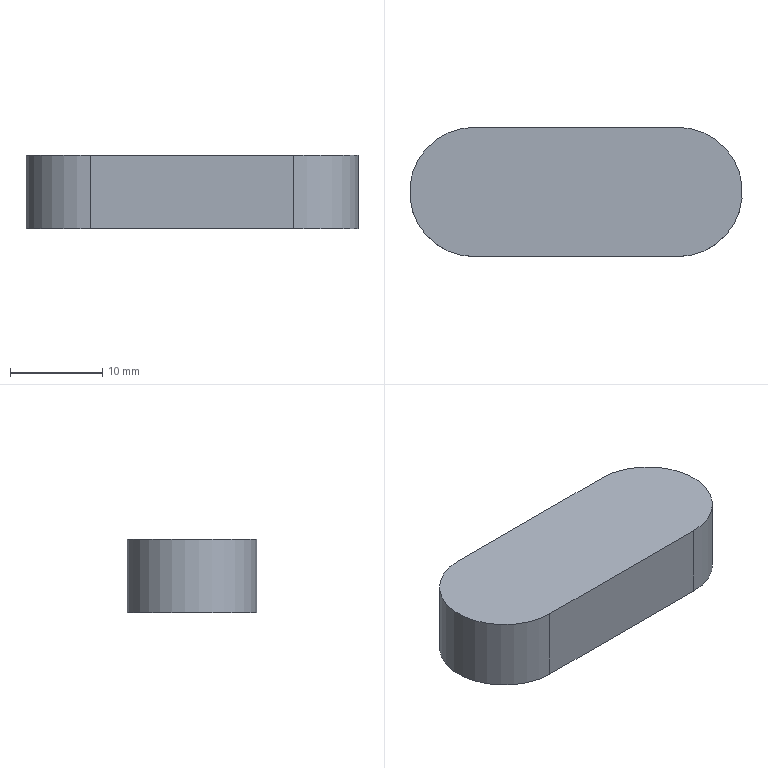Part | NX | features DATUM_CSYS 2, EXTRUDE 1, SKETCH 1 | 1 solid | 6 faces | box 36 x 14 x 8 mm | volume 3696 mm3 | plane 4 | cylinder 2 | commonest cylinder face diameters 14 x2
STEP:
#1=CARTESIAN_POINT('',(-11.,-7.,0.));
#2=VERTEX_POINT('',#1);
#3=CARTESIAN_POINT('',(11.,-7.,0.));
#4=VERTEX_POINT('',#3);
#5=CARTESIAN_POINT('',(-11.,-7.,0.));
#6=DIRECTION('',(1.,0.,0.));
#7=VECTOR('',#6,1000.);
#8=LINE('',#5,#7);
#9=EDGE_CURVE('',#2,#4,#8,.T.);
#10=ORIENTED_EDGE('',*,*,#9,.T.);
#11=CARTESIAN_POINT('',(11.,-7.,8.));
#12=VERTEX_POINT('',#11);
#13=CARTESIAN_POINT('',(11.,-7.,8.));
#14=DIRECTION('',(0.,0.,-1.));
#15=VECTOR('',#14,1000.);
#16=LINE('',#13,#15);
#17=EDGE_CURVE('',#12,#4,#16,.T.);
#18=ORIENTED_EDGE('',*,*,#17,.F.);
#19=CARTESIAN_POINT('',(-11.,-7.,8.));
#20=VERTEX_POINT('',#19);
#21=CARTESIAN_POINT('',(-11.,-7.,8.));
#22=DIRECTION('',(1.,0.,0.));
#23=VECTOR('',#22,1000.);
#24=LINE('',#21,#23);
#25=EDGE_CURVE('',#20,#12,#24,.T.);
#26=ORIENTED_EDGE('',*,*,#25,.F.);
#27=CARTESIAN_POINT('',(-11.,-7.,8.));
#28=DIRECTION('',(0.,0.,-1.));
#29=VECTOR('',#28,1000.);
#30=LINE('',#27,#29);
#31=EDGE_CURVE('',#20,#2,#30,.T.);
#32=ORIENTED_EDGE('',*,*,#31,.T.);
#33=EDGE_LOOP('',(#10,#18,#26,#32));
#34=FACE_BOUND('',#33,.T.);
#35=CARTESIAN_POINT('',(-11.,-7.,8.));
#36=DIRECTION('',(0.,1.,0.));
#37=DIRECTION('',(0.,0.,1.));
#38=AXIS2_PLACEMENT_3D('',#35,#36,#37);
#39=PLANE('',#38);
#40=ADVANCED_FACE('',(#34),#39,.F.);
#41=CARTESIAN_POINT('',(11.,7.,0.));
#42=VERTEX_POINT('',#41);
#43=CARTESIAN_POINT('',(11.,0.,0.));
#44=DIRECTION('',(0.,0.,1.));
#45=DIRECTION('',(-1.,0.,0.));
#46=AXIS2_PLACEMENT_3D('',#43,#44,#45);
#47=CIRCLE('',#46,7.);
#48=EDGE_CURVE('',#4,#42,#47,.T.);
#49=ORIENTED_EDGE('',*,*,#48,.T.);
#50=CARTESIAN_POINT('',(11.,7.,8.));
#51=VERTEX_POINT('',#50);
#52=CARTESIAN_POINT('',(11.,7.,8.));
#53=DIRECTION('',(0.,0.,-1.));
#54=VECTOR('',#53,1000.);
#55=LINE('',#52,#54);
#56=EDGE_CURVE('',#51,#42,#55,.T.);
#57=ORIENTED_EDGE('',*,*,#56,.F.);
#58=CARTESIAN_POINT('',(11.,0.,8.));
#59=DIRECTION('',(0.,0.,1.));
#60=DIRECTION('',(-1.,0.,0.));
#61=AXIS2_PLACEMENT_3D('',#58,#59,#60);
#62=CIRCLE('',#61,7.);
#63=EDGE_CURVE('',#12,#51,#62,.T.);
#64=ORIENTED_EDGE('',*,*,#63,.F.);
#65=ORIENTED_EDGE('',*,*,#17,.T.);
#66=EDGE_LOOP('',(#49,#57,#64,#65));
#67=FACE_BOUND('',#66,.T.);
#68=CARTESIAN_POINT('',(11.,0.,8.));
#69=DIRECTION('',(0.,0.,-1.));
#70=DIRECTION('',(-1.,0.,0.));
#71=AXIS2_PLACEMENT_3D('',#68,#69,#70);
#72=CYLINDRICAL_SURFACE('',#71,7.);
#73=ADVANCED_FACE('',(#67),#72,.T.);
#74=CARTESIAN_POINT('',(-11.,7.,0.));
#75=VERTEX_POINT('',#74);
#76=CARTESIAN_POINT('',(11.,7.,0.));
#77=DIRECTION('',(-1.,0.,0.));
#78=VECTOR('',#77,1000.);
#79=LINE('',#76,#78);
#80=EDGE_CURVE('',#42,#75,#79,.T.);
#81=ORIENTED_EDGE('',*,*,#80,.T.);
#82=CARTESIAN_POINT('',(-11.,7.,8.));
#83=VERTEX_POINT('',#82);
#84=CARTESIAN_POINT('',(-11.,7.,8.));
#85=DIRECTION('',(0.,0.,-1.));
#86=VECTOR('',#85,1000.);
#87=LINE('',#84,#86);
#88=EDGE_CURVE('',#83,#75,#87,.T.);
#89=ORIENTED_EDGE('',*,*,#88,.F.);
#90=CARTESIAN_POINT('',(11.,7.,8.));
#91=DIRECTION('',(-1.,0.,0.));
#92=VECTOR('',#91,1000.);
#93=LINE('',#90,#92);
#94=EDGE_CURVE('',#51,#83,#93,.T.);
#95=ORIENTED_EDGE('',*,*,#94,.F.);
#96=ORIENTED_EDGE('',*,*,#56,.T.);
#97=EDGE_LOOP('',(#81,#89,#95,#96));
#98=FACE_BOUND('',#97,.T.);
#99=CARTESIAN_POINT('',(11.,7.,8.));
#100=DIRECTION('',(0.,-1.,0.));
#101=DIRECTION('',(0.,0.,-1.));
#102=AXIS2_PLACEMENT_3D('',#99,#100,#101);
#103=PLANE('',#102);
#104=ADVANCED_FACE('',(#98),#103,.F.);
#105=CARTESIAN_POINT('',(-11.,0.,0.));
#106=DIRECTION('',(0.,0.,1.));
#107=DIRECTION('',(1.,0.,0.));
#108=AXIS2_PLACEMENT_3D('',#105,#106,#107);
#109=CIRCLE('',#108,7.);
#110=EDGE_CURVE('',#75,#2,#109,.T.);
#111=ORIENTED_EDGE('',*,*,#110,.T.);
#112=ORIENTED_EDGE('',*,*,#31,.F.);
#113=CARTESIAN_POINT('',(-11.,0.,8.));
#114=DIRECTION('',(0.,0.,1.));
#115=DIRECTION('',(1.,0.,0.));
#116=AXIS2_PLACEMENT_3D('',#113,#114,#115);
#117=CIRCLE('',#116,7.);
#118=EDGE_CURVE('',#83,#20,#117,.T.);
#119=ORIENTED_EDGE('',*,*,#118,.F.);
#120=ORIENTED_EDGE('',*,*,#88,.T.);
#121=EDGE_LOOP('',(#111,#112,#119,#120));
#122=FACE_BOUND('',#121,.T.);
#123=CARTESIAN_POINT('',(-11.,0.,8.));
#124=DIRECTION('',(0.,0.,-1.));
#125=DIRECTION('',(-1.,0.,0.));
#126=AXIS2_PLACEMENT_3D('',#123,#124,#125);
#127=CYLINDRICAL_SURFACE('',#126,7.);
#128=ADVANCED_FACE('',(#122),#127,.T.);
#129=ORIENTED_EDGE('',*,*,#25,.T.);
#130=ORIENTED_EDGE('',*,*,#63,.T.);
#131=ORIENTED_EDGE('',*,*,#94,.T.);
#132=ORIENTED_EDGE('',*,*,#118,.T.);
#133=EDGE_LOOP('',(#129,#130,#131,#132));
#134=FACE_BOUND('',#133,.T.);
#135=CARTESIAN_POINT('',(11.,0.,8.));
#136=DIRECTION('',(0.,0.,1.));
#137=DIRECTION('',(1.,0.,0.));
#138=AXIS2_PLACEMENT_3D('',#135,#136,#137);
#139=PLANE('',#138);
#140=ADVANCED_FACE('',(#134),#139,.T.);
#141=ORIENTED_EDGE('',*,*,#9,.F.);
#142=ORIENTED_EDGE('',*,*,#110,.F.);
#143=ORIENTED_EDGE('',*,*,#80,.F.);
#144=ORIENTED_EDGE('',*,*,#48,.F.);
#145=EDGE_LOOP('',(#141,#142,#143,#144));
#146=FACE_BOUND('',#145,.T.);
#147=CARTESIAN_POINT('',(11.,0.,0.));
#148=DIRECTION('',(0.,0.,1.));
#149=DIRECTION('',(1.,0.,0.));
#150=AXIS2_PLACEMENT_3D('',#147,#148,#149);
#151=PLANE('',#150);
#152=ADVANCED_FACE('',(#146),#151,.F.);
#153=CLOSED_SHELL('',(#40,#73,#104,#128,#140,#152));
#154=MANIFOLD_SOLID_BREP('',#153);
#155=(LENGTH_UNIT()NAMED_UNIT(*)SI_UNIT(.MILLI.,.METRE.));
#156=UNCERTAINTY_MEASURE_WITH_UNIT(LENGTH_MEASURE(0.00001),#155,'','');
#157=(NAMED_UNIT(*)PLANE_ANGLE_UNIT()SI_UNIT($,.RADIAN.));
#158=(NAMED_UNIT(*)SI_UNIT($,.STERADIAN.)SOLID_ANGLE_UNIT());
#159=(GEOMETRIC_REPRESENTATION_CONTEXT(3)GLOBAL_UNCERTAINTY_ASSIGNED_CONTEXT((#156))GLOBAL_UNIT_ASSIGNED_CONTEXT((#155,#157,#158))REPRESENTATION_CONTEXT('',''));
#160=ADVANCED_BREP_SHAPE_REPRESENTATION('',(#154),#159);